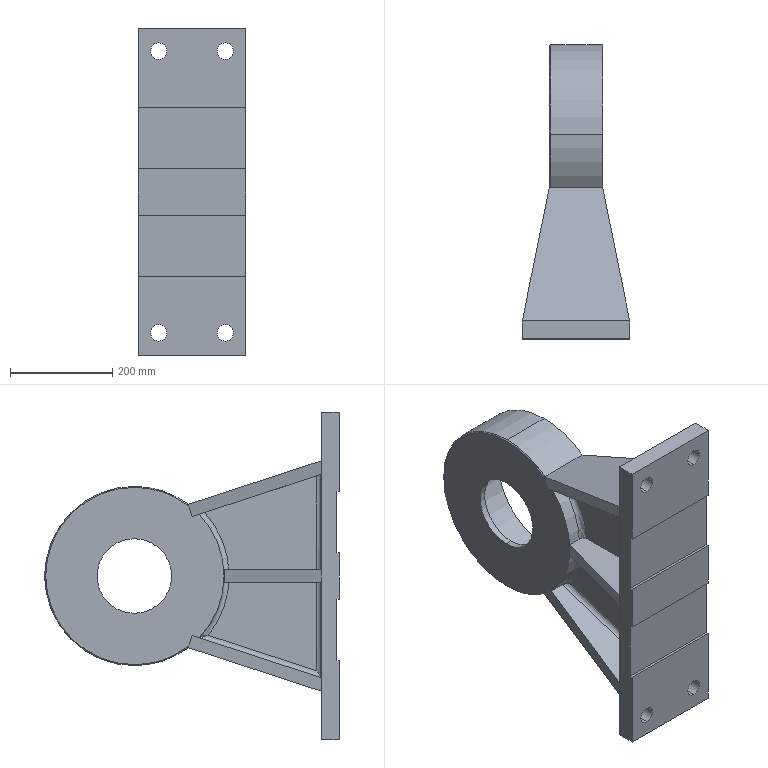Part | SolidWorks | features ICE 5, HoleWzd 2, 3DProfileFeature 1, Chamfer 1, Fillet 1, MirrorPattern 1, Revolution 1 | 2 solids | 94 faces | box 210 x 575 x 640 mm | volume 14558627 mm3 | plane 39 | cylinder 38 | cone 15 | torus 2 | commonest cylinder face diameters 14 x12 32 x8 20 x5 350 x5 14.5 x2 146 x2